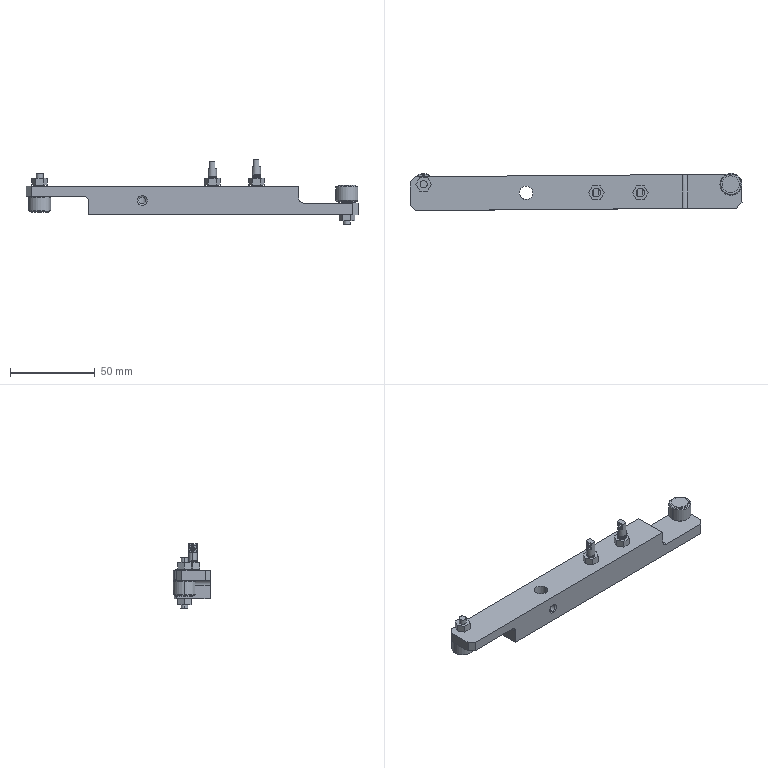Part | NX | 9 solids | 218 faces | box 196.107 x 22.03 x 38 mm | volume 54101 mm3 | cylinder 104 | plane 72 | cone 26 | spline 16 | commonest cylinder face diameters 5 x66 4.2 x18 10 x8 2 x4 13 x4 6 x2